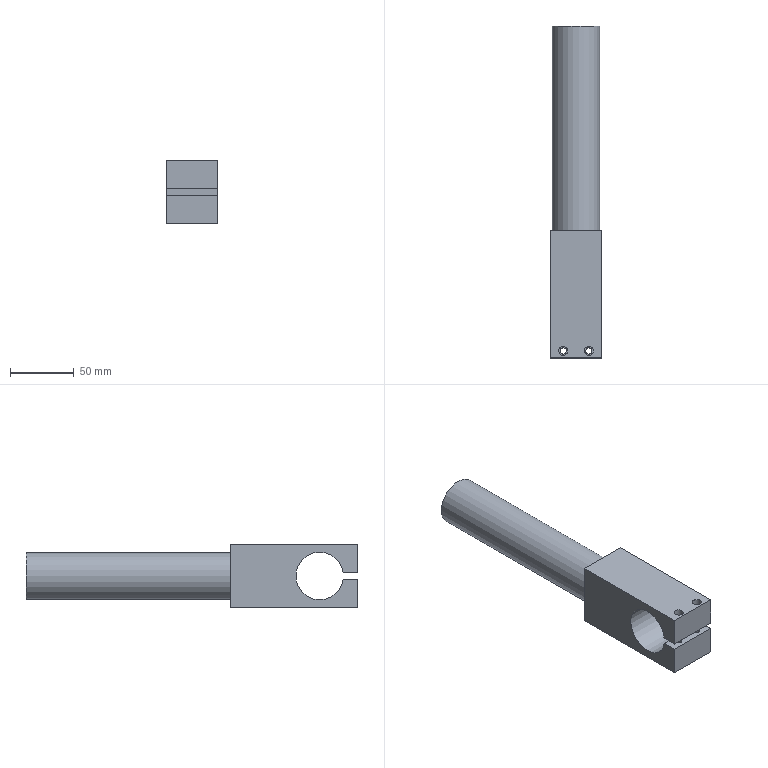Part | STEP file | SN10_010_001_SUPORTE | 1 solid | 16 faces | box 40 x 260 x 50 mm | volume 323681 mm3 | plane 10 | cylinder 6 | commonest cylinder face diameters 4.917 x2 7 x2 37 x1 37.2 x1
STEP:
#1=CARTESIAN_POINT('',(0.,0.,0.));
#2=DIRECTION('',(0.,0.,1.));
#3=DIRECTION('',(1.,0.,0.));
#4=AXIS2_PLACEMENT_3D('',#1,#2,#3);
#5=CARTESIAN_POINT('',(6.928,-22.822,2.5));
#6=VERTEX_POINT('',#5);
#7=CARTESIAN_POINT('',(10.,-24.5,2.5));
#8=DIRECTION('',(0.,0.,-1.));
#9=DIRECTION('',(1.,0.,0.));
#10=AXIS2_PLACEMENT_3D('',#7,#8,#9);
#11=CIRCLE('',#10,3.5);
#12=CARTESIAN_POINT('',(10.,-24.5,24.9));
#13=DIRECTION('',(0.,0.,-1.));
#14=DIRECTION('',(0.8776,-0.4794,0.));
#15=AXIS2_PLACEMENT_3D('',#12,#13,#14);
#16=CYLINDRICAL_SURFACE('',#15,3.5);
#17=CARTESIAN_POINT('',(-0.5,22.4));
#18=DIRECTION('',(1.,0.));
#19=VECTOR('',#18,1.);
#20=LINE('',#17,#19);
#21=(GEOMETRIC_REPRESENTATION_CONTEXT(2)PARAMETRIC_REPRESENTATION_CONTEXT()REPRESENTATION_CONTEXT('',''));
#22=DEFINITIONAL_REPRESENTATION('',(#20),#21);
#23=PCURVE('',#16,#22);
#24=CARTESIAN_POINT('',(20.,-30.,2.5));
#25=DIRECTION('',(0.,0.,1.));
#26=DIRECTION('',(1.,0.,0.));
#27=AXIS2_PLACEMENT_3D('',#24,#25,#26);
#28=PLANE('',#27);
#29=CARTESIAN_POINT('',(-6.5,5.5));
#30=CARTESIAN_POINT('',(-6.5,-0.5622));
#31=CARTESIAN_POINT('',(-11.75,2.469));
#32=CARTESIAN_POINT('',(-17.,5.5));
#33=CARTESIAN_POINT('',(-11.75,8.531));
#34=CARTESIAN_POINT('',(-6.5,11.562));
#35=CARTESIAN_POINT('',(-6.5,5.5));
#36=(BOUNDED_CURVE()B_SPLINE_CURVE(2,(#29,#30,#31,#32,#33,#34,#35),.UNSPECIFIED.,.T.,.F.)B_SPLINE_CURVE_WITH_KNOTS((1,2,2,2,2,1),(-2.094,0.,2.094,4.189,6.283,8.378),.UNSPECIFIED.)CURVE()GEOMETRIC_REPRESENTATION_ITEM()RATIONAL_B_SPLINE_CURVE((1.,0.5,1.,0.5,1.,0.5,1.))REPRESENTATION_ITEM(''));
#37=(GEOMETRIC_REPRESENTATION_CONTEXT(2)PARAMETRIC_REPRESENTATION_CONTEXT()REPRESENTATION_CONTEXT('',''));
#38=DEFINITIONAL_REPRESENTATION('',(#36),#37);
#39=PCURVE('',#28,#38);
#40=SURFACE_CURVE('',#11,(#23,#39),.PCURVE_S1.);
#41=EDGE_CURVE('',#6,#6,#40,.T.);
#42=ORIENTED_EDGE('',*,*,#41,.F.);
#43=CARTESIAN_POINT('',(6.928,-22.822,25.));
#44=VERTEX_POINT('',#43);
#45=CARTESIAN_POINT('',(6.928,-22.822,25.));
#46=CARTESIAN_POINT('',(6.928,-22.822,2.5));
#47=B_SPLINE_CURVE_WITH_KNOTS('',1,(#45,#46),.UNSPECIFIED.,.F.,.F.,(2,2),(-0.1,22.4),.PIECEWISE_BEZIER_KNOTS.);
#48=CARTESIAN_POINT('',(3.142,0.));
#49=DIRECTION('',(0.,1.));
#50=VECTOR('',#49,1.);
#51=LINE('',#48,#50);
#52=(GEOMETRIC_REPRESENTATION_CONTEXT(2)PARAMETRIC_REPRESENTATION_CONTEXT()REPRESENTATION_CONTEXT('',''));
#53=DEFINITIONAL_REPRESENTATION('',(#51),#52);
#54=PCURVE('',#16,#53);
#55=CARTESIAN_POINT('',(9.425,0.));
#56=DIRECTION('',(0.,1.));
#57=VECTOR('',#56,1.);
#58=LINE('',#55,#57);
#59=(GEOMETRIC_REPRESENTATION_CONTEXT(2)PARAMETRIC_REPRESENTATION_CONTEXT()REPRESENTATION_CONTEXT('',''));
#60=DEFINITIONAL_REPRESENTATION('',(#58),#59);
#61=PCURVE('',#16,#60);
#62=SEAM_CURVE('',#47,(#54,#61),.PCURVE_S1.);
#63=EDGE_CURVE('',#44,#6,#62,.T.);
#64=ORIENTED_EDGE('',*,*,#63,.F.);
#65=CARTESIAN_POINT('',(10.,-24.5,25.));
#66=DIRECTION('',(0.,0.,-1.));
#67=DIRECTION('',(1.,0.,0.));
#68=AXIS2_PLACEMENT_3D('',#65,#66,#67);
#69=CIRCLE('',#68,3.5);
#70=CARTESIAN_POINT('',(-0.5,-0.1));
#71=DIRECTION('',(1.,0.));
#72=VECTOR('',#71,1.);
#73=LINE('',#70,#72);
#74=(GEOMETRIC_REPRESENTATION_CONTEXT(2)PARAMETRIC_REPRESENTATION_CONTEXT()REPRESENTATION_CONTEXT('',''));
#75=DEFINITIONAL_REPRESENTATION('',(#73),#74);
#76=PCURVE('',#16,#75);
#77=CARTESIAN_POINT('',(0.,-30.,25.));
#78=DIRECTION('',(0.,0.,-1.));
#79=DIRECTION('',(-1.,0.,0.));
#80=AXIS2_PLACEMENT_3D('',#77,#78,#79);
#81=PLANE('',#80);
#82=CARTESIAN_POINT('',(-10.,5.5));
#83=DIRECTION('',(-1.,0.));
#84=AXIS2_PLACEMENT_2D('',#82,#83);
#85=CIRCLE('',#84,3.5);
#86=(GEOMETRIC_REPRESENTATION_CONTEXT(2)PARAMETRIC_REPRESENTATION_CONTEXT()REPRESENTATION_CONTEXT('',''));
#87=DEFINITIONAL_REPRESENTATION('',(#85),#86);
#88=PCURVE('',#81,#87);
#89=SURFACE_CURVE('',#69,(#76,#88),.PCURVE_S1.);
#90=EDGE_CURVE('',#44,#44,#89,.T.);
#91=ORIENTED_EDGE('',*,*,#90,.T.);
#92=ORIENTED_EDGE('',*,*,#63,.T.);
#93=EDGE_LOOP('',(#42,#64,#91,#92));
#94=FACE_BOUND('',#93,.F.);
#95=ADVANCED_FACE('',(#94),#16,.F.);
#96=CARTESIAN_POINT('',(20.,-30.,25.));
#97=VERTEX_POINT('',#96);
#98=CARTESIAN_POINT('',(20.,-30.,2.5));
#99=VERTEX_POINT('',#98);
#100=CARTESIAN_POINT('',(20.,-30.,25.));
#101=DIRECTION('',(0.,0.,-1.));
#102=VECTOR('',#101,1.);
#103=LINE('',#100,#102);
#104=CARTESIAN_POINT('',(0.,-30.,25.));
#105=DIRECTION('',(0.,-1.,0.));
#106=DIRECTION('',(0.,0.,-1.));
#107=AXIS2_PLACEMENT_3D('',#104,#105,#106);
#108=PLANE('',#107);
#109=CARTESIAN_POINT('',(0.,20.));
#110=DIRECTION('',(1.,0.));
#111=VECTOR('',#110,1.);
#112=LINE('',#109,#111);
#113=(GEOMETRIC_REPRESENTATION_CONTEXT(2)PARAMETRIC_REPRESENTATION_CONTEXT()REPRESENTATION_CONTEXT('',''));
#114=DEFINITIONAL_REPRESENTATION('',(#112),#113);
#115=PCURVE('',#108,#114);
#116=CARTESIAN_POINT('',(20.,0.,0.));
#117=DIRECTION('',(1.,0.,0.));
#118=DIRECTION('',(0.,0.,-1.));
#119=AXIS2_PLACEMENT_3D('',#116,#117,#118);
#120=PLANE('',#119);
#121=CARTESIAN_POINT('',(-25.,-30.));
#122=DIRECTION('',(1.,0.));
#123=VECTOR('',#122,1.);
#124=LINE('',#121,#123);
#125=(GEOMETRIC_REPRESENTATION_CONTEXT(2)PARAMETRIC_REPRESENTATION_CONTEXT()REPRESENTATION_CONTEXT('',''));
#126=DEFINITIONAL_REPRESENTATION('',(#124),#125);
#127=PCURVE('',#120,#126);
#128=SURFACE_CURVE('',#103,(#115,#127),.PCURVE_S1.);
#129=EDGE_CURVE('',#97,#99,#128,.T.);
#130=ORIENTED_EDGE('',*,*,#129,.F.);
#131=CARTESIAN_POINT('',(-20.,-30.,25.));
#132=VERTEX_POINT('',#131);
#133=CARTESIAN_POINT('',(-20.,-30.,25.));
#134=DIRECTION('',(1.,0.,0.));
#135=VECTOR('',#134,1.);
#136=LINE('',#133,#135);
#137=CARTESIAN_POINT('',(0.,-20.));
#138=DIRECTION('',(0.,1.));
#139=VECTOR('',#138,1.);
#140=LINE('',#137,#139);
#141=(GEOMETRIC_REPRESENTATION_CONTEXT(2)PARAMETRIC_REPRESENTATION_CONTEXT()REPRESENTATION_CONTEXT('',''));
#142=DEFINITIONAL_REPRESENTATION('',(#140),#141);
#143=PCURVE('',#108,#142);
#144=CARTESIAN_POINT('',(20.,0.));
#145=DIRECTION('',(-1.,0.));
#146=VECTOR('',#145,1.);
#147=LINE('',#144,#146);
#148=(GEOMETRIC_REPRESENTATION_CONTEXT(2)PARAMETRIC_REPRESENTATION_CONTEXT()REPRESENTATION_CONTEXT('',''));
#149=DEFINITIONAL_REPRESENTATION('',(#147),#148);
#150=PCURVE('',#81,#149);
#151=SURFACE_CURVE('',#136,(#143,#150),.PCURVE_S1.);
#152=EDGE_CURVE('',#132,#97,#151,.T.);
#153=ORIENTED_EDGE('',*,*,#152,.F.);
#154=CARTESIAN_POINT('',(-20.,-30.,2.5));
#155=VERTEX_POINT('',#154);
#156=CARTESIAN_POINT('',(-20.,-30.,25.));
#157=DIRECTION('',(0.,0.,-1.));
#158=VECTOR('',#157,1.);
#159=LINE('',#156,#158);
#160=CARTESIAN_POINT('',(0.,-20.));
#161=DIRECTION('',(1.,0.));
#162=VECTOR('',#161,1.);
#163=LINE('',#160,#162);
#164=(GEOMETRIC_REPRESENTATION_CONTEXT(2)PARAMETRIC_REPRESENTATION_CONTEXT()REPRESENTATION_CONTEXT('',''));
#165=DEFINITIONAL_REPRESENTATION('',(#163),#164);
#166=PCURVE('',#108,#165);
#167=CARTESIAN_POINT('',(-20.,0.,0.));
#168=DIRECTION('',(1.,0.,0.));
#169=DIRECTION('',(0.,0.,-1.));
#170=AXIS2_PLACEMENT_3D('',#167,#168,#169);
#171=PLANE('',#170);
#172=CARTESIAN_POINT('',(-25.,-30.));
#173=DIRECTION('',(1.,0.));
#174=VECTOR('',#173,1.);
#175=LINE('',#172,#174);
#176=(GEOMETRIC_REPRESENTATION_CONTEXT(2)PARAMETRIC_REPRESENTATION_CONTEXT()REPRESENTATION_CONTEXT('',''));
#177=DEFINITIONAL_REPRESENTATION('',(#175),#176);
#178=PCURVE('',#171,#177);
#179=SURFACE_CURVE('',#159,(#166,#178),.PCURVE_S1.);
#180=EDGE_CURVE('',#132,#155,#179,.T.);
#181=ORIENTED_EDGE('',*,*,#180,.T.);
#182=CARTESIAN_POINT('',(20.,-30.,2.5));
#183=DIRECTION('',(-1.,0.,0.));
#184=VECTOR('',#183,1.);
#185=LINE('',#182,#184);
#186=CARTESIAN_POINT('',(22.5,20.));
#187=DIRECTION('',(0.,-1.));
#188=VECTOR('',#187,1.);
#189=LINE('',#186,#188);
#190=(GEOMETRIC_REPRESENTATION_CONTEXT(2)PARAMETRIC_REPRESENTATION_CONTEXT()REPRESENTATION_CONTEXT('',''));
#191=DEFINITIONAL_REPRESENTATION('',(#189),#190);
#192=PCURVE('',#108,#191);
#193=CARTESIAN_POINT('',(0.,0.));
#194=DIRECTION('',(-1.,0.));
#195=VECTOR('',#194,1.);
#196=LINE('',#193,#195);
#197=(GEOMETRIC_REPRESENTATION_CONTEXT(2)PARAMETRIC_REPRESENTATION_CONTEXT()REPRESENTATION_CONTEXT('',''));
#198=DEFINITIONAL_REPRESENTATION('',(#196),#197);
#199=PCURVE('',#28,#198);
#200=SURFACE_CURVE('',#185,(#192,#199),.PCURVE_S1.);
#201=EDGE_CURVE('',#99,#155,#200,.T.);
#202=ORIENTED_EDGE('',*,*,#201,.F.);
#203=EDGE_LOOP('',(#130,#153,#181,#202));
#204=FACE_BOUND('',#203,.T.);
#205=ADVANCED_FACE('',(#204),#108,.T.);
#206=CARTESIAN_POINT('',(20.,-30.,-2.5));
#207=VERTEX_POINT('',#206);
#208=CARTESIAN_POINT('',(20.,-30.,-25.));
#209=VERTEX_POINT('',#208);
#210=CARTESIAN_POINT('',(20.,-30.,-2.5));
#211=DIRECTION('',(0.,0.,-1.));
#212=VECTOR('',#211,1.);
#213=LINE('',#210,#212);
#214=CARTESIAN_POINT('',(2.5,-30.));
#215=DIRECTION('',(1.,0.));
#216=VECTOR('',#215,1.);
#217=LINE('',#214,#216);
#218=(GEOMETRIC_REPRESENTATION_CONTEXT(2)PARAMETRIC_REPRESENTATION_CONTEXT()REPRESENTATION_CONTEXT('',''));
#219=DEFINITIONAL_REPRESENTATION('',(#217),#218);
#220=PCURVE('',#120,#219);
#221=CARTESIAN_POINT('',(0.,-30.,25.));
#222=DIRECTION('',(0.,-1.,0.));
#223=DIRECTION('',(0.,0.,-1.));
#224=AXIS2_PLACEMENT_3D('',#221,#222,#223);
#225=PLANE('',#224);
#226=CARTESIAN_POINT('',(27.5,20.));
#227=DIRECTION('',(1.,0.));
#228=VECTOR('',#227,1.);
#229=LINE('',#226,#228);
#230=(GEOMETRIC_REPRESENTATION_CONTEXT(2)PARAMETRIC_REPRESENTATION_CONTEXT()REPRESENTATION_CONTEXT('',''));
#231=DEFINITIONAL_REPRESENTATION('',(#229),#230);
#232=PCURVE('',#225,#231);
#233=SURFACE_CURVE('',#213,(#220,#232),.PCURVE_S1.);
#234=EDGE_CURVE('',#207,#209,#233,.T.);
#235=ORIENTED_EDGE('',*,*,#234,.T.);
#236=CARTESIAN_POINT('',(20.,70.,-25.));
#237=VERTEX_POINT('',#236);
#238=CARTESIAN_POINT('',(20.,70.,-25.));
#239=DIRECTION('',(0.,-1.,0.));
#240=VECTOR('',#239,1.);
#241=LINE('',#238,#240);
#242=CARTESIAN_POINT('',(25.,70.));
#243=DIRECTION('',(0.,-1.));
#244=VECTOR('',#243,1.);
#245=LINE('',#242,#244);
#246=(GEOMETRIC_REPRESENTATION_CONTEXT(2)PARAMETRIC_REPRESENTATION_CONTEXT()REPRESENTATION_CONTEXT('',''));
#247=DEFINITIONAL_REPRESENTATION('',(#245),#246);
#248=PCURVE('',#120,#247);
#249=CARTESIAN_POINT('',(0.,70.,-25.));
#250=DIRECTION('',(0.,0.,1.));
#251=DIRECTION('',(1.,0.,0.));
#252=AXIS2_PLACEMENT_3D('',#249,#250,#251);
#253=PLANE('',#252);
#254=CARTESIAN_POINT('',(20.,0.));
#255=DIRECTION('',(0.,-1.));
#256=VECTOR('',#255,1.);
#257=LINE('',#254,#256);
#258=(GEOMETRIC_REPRESENTATION_CONTEXT(2)PARAMETRIC_REPRESENTATION_CONTEXT()REPRESENTATION_CONTEXT('',''));
#259=DEFINITIONAL_REPRESENTATION('',(#257),#258);
#260=PCURVE('',#253,#259);
#261=SURFACE_CURVE('',#241,(#248,#260),.PCURVE_S1.);
#262=EDGE_CURVE('',#237,#209,#261,.T.);
#263=ORIENTED_EDGE('',*,*,#262,.F.);
#264=CARTESIAN_POINT('',(20.,70.,25.));
#265=VERTEX_POINT('',#264);
#266=CARTESIAN_POINT('',(20.,70.,-25.));
#267=DIRECTION('',(0.,0.,1.));
#268=VECTOR('',#267,1.);
#269=LINE('',#266,#268);
#270=CARTESIAN_POINT('',(25.,70.));
#271=DIRECTION('',(-1.,0.));
#272=VECTOR('',#271,1.);
#273=LINE('',#270,#272);
#274=(GEOMETRIC_REPRESENTATION_CONTEXT(2)PARAMETRIC_REPRESENTATION_CONTEXT()REPRESENTATION_CONTEXT('',''));
#275=DEFINITIONAL_REPRESENTATION('',(#273),#274);
#276=PCURVE('',#120,#275);
#277=CARTESIAN_POINT('',(0.,70.,-25.));
#278=DIRECTION('',(0.,1.,0.));
#279=DIRECTION('',(0.,0.,1.));
#280=AXIS2_PLACEMENT_3D('',#277,#278,#279);
#281=PLANE('',#280);
#282=CARTESIAN_POINT('',(0.,20.));
#283=DIRECTION('',(1.,0.));
#284=VECTOR('',#283,1.);
#285=LINE('',#282,#284);
#286=(GEOMETRIC_REPRESENTATION_CONTEXT(2)PARAMETRIC_REPRESENTATION_CONTEXT()REPRESENTATION_CONTEXT('',''));
#287=DEFINITIONAL_REPRESENTATION('',(#285),#286);
#288=PCURVE('',#281,#287);
#289=SURFACE_CURVE('',#269,(#276,#288),.PCURVE_S1.);
#290=EDGE_CURVE('',#237,#265,#289,.T.);
#291=ORIENTED_EDGE('',*,*,#290,.T.);
#292=CARTESIAN_POINT('',(20.,-30.,25.));
#293=DIRECTION('',(0.,1.,0.));
#294=VECTOR('',#293,1.);
#295=LINE('',#292,#294);
#296=CARTESIAN_POINT('',(-25.,-30.));
#297=DIRECTION('',(0.,1.));
#298=VECTOR('',#297,1.);
#299=LINE('',#296,#298);
#300=(GEOMETRIC_REPRESENTATION_CONTEXT(2)PARAMETRIC_REPRESENTATION_CONTEXT()REPRESENTATION_CONTEXT('',''));
#301=DEFINITIONAL_REPRESENTATION('',(#299),#300);
#302=PCURVE('',#120,#301);
#303=CARTESIAN_POINT('',(-20.,0.));
#304=DIRECTION('',(0.,1.));
#305=VECTOR('',#304,1.);
#306=LINE('',#303,#305);
#307=(GEOMETRIC_REPRESENTATION_CONTEXT(2)PARAMETRIC_REPRESENTATION_CONTEXT()REPRESENTATION_CONTEXT('',''));
#308=DEFINITIONAL_REPRESENTATION('',(#306),#307);
#309=PCURVE('',#81,#308);
#310=SURFACE_CURVE('',#295,(#302,#309),.PCURVE_S1.);
#311=EDGE_CURVE('',#97,#265,#310,.T.);
#312=ORIENTED_EDGE('',*,*,#311,.F.);
#313=ORIENTED_EDGE('',*,*,#129,.T.);
#314=CARTESIAN_POINT('',(20.,-18.431,2.5));
#315=VERTEX_POINT('',#314);
#316=CARTESIAN_POINT('',(20.,-30.,2.5));
#317=DIRECTION('',(0.,1.,0.));
#318=VECTOR('',#317,1.);
#319=LINE('',#316,#318);
#320=CARTESIAN_POINT('',(-2.5,-30.));
#321=DIRECTION('',(0.,1.));
#322=VECTOR('',#321,1.);
#323=LINE('',#320,#322);
#324=(GEOMETRIC_REPRESENTATION_CONTEXT(2)PARAMETRIC_REPRESENTATION_CONTEXT()REPRESENTATION_CONTEXT('',''));
#325=DEFINITIONAL_REPRESENTATION('',(#323),#324);
#326=PCURVE('',#120,#325);
#327=CARTESIAN_POINT('',(0.,0.));
#328=DIRECTION('',(0.,1.));
#329=VECTOR('',#328,1.);
#330=LINE('',#327,#329);
#331=(GEOMETRIC_REPRESENTATION_CONTEXT(2)PARAMETRIC_REPRESENTATION_CONTEXT()REPRESENTATION_CONTEXT('',''));
#332=DEFINITIONAL_REPRESENTATION('',(#330),#331);
#333=PCURVE('',#28,#332);
#334=SURFACE_CURVE('',#319,(#326,#333),.PCURVE_S1.);
#335=EDGE_CURVE('',#99,#315,#334,.T.);
#336=ORIENTED_EDGE('',*,*,#335,.T.);
#337=CARTESIAN_POINT('',(20.,-18.431,-2.5));
#338=VERTEX_POINT('',#337);
#339=CARTESIAN_POINT('',(20.,0.,0.));
#340=DIRECTION('',(1.,0.,0.));
#341=DIRECTION('',(0.,1.,0.));
#342=AXIS2_PLACEMENT_3D('',#339,#340,#341);
#343=CIRCLE('',#342,18.6);
#344=CARTESIAN_POINT('',(0.,0.));
#345=DIRECTION('',(0.,1.));
#346=AXIS2_PLACEMENT_2D('',#344,#345);
#347=CIRCLE('',#346,18.6);
#348=(GEOMETRIC_REPRESENTATION_CONTEXT(2)PARAMETRIC_REPRESENTATION_CONTEXT()REPRESENTATION_CONTEXT('',''));
#349=DEFINITIONAL_REPRESENTATION('',(#347),#348);
#350=PCURVE('',#120,#349);
#351=CARTESIAN_POINT('',(19.9,0.,0.));
#352=DIRECTION('',(-1.,0.,0.));
#353=DIRECTION('',(0.,0.8776,-0.4794));
#354=AXIS2_PLACEMENT_3D('',#351,#352,#353);
#355=CYLINDRICAL_SURFACE('',#354,18.6);
#356=CARTESIAN_POINT('',(12.066,-0.1));
#357=DIRECTION('',(-1.,0.));
#358=VECTOR('',#357,1.);
#359=LINE('',#356,#358);
#360=(GEOMETRIC_REPRESENTATION_CONTEXT(2)PARAMETRIC_REPRESENTATION_CONTEXT()REPRESENTATION_CONTEXT('',''));
#361=DEFINITIONAL_REPRESENTATION('',(#359),#360);
#362=PCURVE('',#355,#361);
#363=SURFACE_CURVE('',#343,(#350,#362),.PCURVE_S1.);
#364=EDGE_CURVE('',#338,#315,#363,.T.);
#365=ORIENTED_EDGE('',*,*,#364,.F.);
#366=CARTESIAN_POINT('',(20.,-18.431,-2.5));
#367=DIRECTION('',(0.,-1.,0.));
#368=VECTOR('',#367,1.);
#369=LINE('',#366,#368);
#370=CARTESIAN_POINT('',(2.5,-18.431));
#371=DIRECTION('',(0.,-1.));
#372=VECTOR('',#371,1.);
#373=LINE('',#370,#372);
#374=(GEOMETRIC_REPRESENTATION_CONTEXT(2)PARAMETRIC_REPRESENTATION_CONTEXT()REPRESENTATION_CONTEXT('',''));
#375=DEFINITIONAL_REPRESENTATION('',(#373),#374);
#376=PCURVE('',#120,#375);
#377=CARTESIAN_POINT('',(20.,-18.431,-2.5));
#378=DIRECTION('',(0.,0.,-1.));
#379=DIRECTION('',(-1.,0.,0.));
#380=AXIS2_PLACEMENT_3D('',#377,#378,#379);
#381=PLANE('',#380);
#382=CARTESIAN_POINT('',(0.,0.));
#383=DIRECTION('',(0.,-1.));
#384=VECTOR('',#383,1.);
#385=LINE('',#382,#384);
#386=(GEOMETRIC_REPRESENTATION_CONTEXT(2)PARAMETRIC_REPRESENTATION_CONTEXT()REPRESENTATION_CONTEXT('',''));
#387=DEFINITIONAL_REPRESENTATION('',(#385),#386);
#388=PCURVE('',#381,#387);
#389=SURFACE_CURVE('',#369,(#376,#388),.PCURVE_S1.);
#390=EDGE_CURVE('',#338,#207,#389,.T.);
#391=ORIENTED_EDGE('',*,*,#390,.T.);
#392=EDGE_LOOP('',(#235,#263,#291,#312,#313,#336,#365,#391));
#393=FACE_BOUND('',#392,.T.);
#394=ADVANCED_FACE('',(#393),#120,.T.);
#395=CARTESIAN_POINT('',(-20.,-30.,-2.5));
#396=VERTEX_POINT('',#395);
#397=CARTESIAN_POINT('',(-20.,-18.431,-2.5));
#398=VERTEX_POINT('',#397);
#399=CARTESIAN_POINT('',(-20.,-30.,-2.5));
#400=DIRECTION('',(0.,1.,0.));
#401=VECTOR('',#400,1.);
#402=LINE('',#399,#401);
#403=CARTESIAN_POINT('',(2.5,-30.));
#404=DIRECTION('',(0.,1.));
#405=VECTOR('',#404,1.);
#406=LINE('',#403,#405);
#407=(GEOMETRIC_REPRESENTATION_CONTEXT(2)PARAMETRIC_REPRESENTATION_CONTEXT()REPRESENTATION_CONTEXT('',''));
#408=DEFINITIONAL_REPRESENTATION('',(#406),#407);
#409=PCURVE('',#171,#408);
#410=CARTESIAN_POINT('',(40.,-11.569));
#411=DIRECTION('',(0.,1.));
#412=VECTOR('',#411,1.);
#413=LINE('',#410,#412);
#414=(GEOMETRIC_REPRESENTATION_CONTEXT(2)PARAMETRIC_REPRESENTATION_CONTEXT()REPRESENTATION_CONTEXT('',''));
#415=DEFINITIONAL_REPRESENTATION('',(#413),#414);
#416=PCURVE('',#381,#415);
#417=SURFACE_CURVE('',#402,(#409,#416),.PCURVE_S1.);
#418=EDGE_CURVE('',#396,#398,#417,.T.);
#419=ORIENTED_EDGE('',*,*,#418,.T.);
#420=CARTESIAN_POINT('',(-20.,-18.431,2.5));
#421=VERTEX_POINT('',#420);
#422=CARTESIAN_POINT('',(-20.,0.,0.));
#423=DIRECTION('',(1.,0.,0.));
#424=DIRECTION('',(0.,1.,0.));
#425=AXIS2_PLACEMENT_3D('',#422,#423,#424);
#426=CIRCLE('',#425,18.6);
#427=CARTESIAN_POINT('',(0.,0.));
#428=DIRECTION('',(0.,1.));
#429=AXIS2_PLACEMENT_2D('',#427,#428);
#430=CIRCLE('',#429,18.6);
#431=(GEOMETRIC_REPRESENTATION_CONTEXT(2)PARAMETRIC_REPRESENTATION_CONTEXT()REPRESENTATION_CONTEXT('',''));
#432=DEFINITIONAL_REPRESENTATION('',(#430),#431);
#433=PCURVE('',#171,#432);
#434=CARTESIAN_POINT('',(12.066,39.9));
#435=DIRECTION('',(-1.,0.));
#436=VECTOR('',#435,1.);
#437=LINE('',#434,#436);
#438=(GEOMETRIC_REPRESENTATION_CONTEXT(2)PARAMETRIC_REPRESENTATION_CONTEXT()REPRESENTATION_CONTEXT('',''));
#439=DEFINITIONAL_REPRESENTATION('',(#437),#438);
#440=PCURVE('',#355,#439);
#441=SURFACE_CURVE('',#426,(#433,#440),.PCURVE_S1.);
#442=EDGE_CURVE('',#398,#421,#441,.T.);
#443=ORIENTED_EDGE('',*,*,#442,.T.);
#444=CARTESIAN_POINT('',(-20.,-30.,2.5));
#445=DIRECTION('',(0.,1.,0.));
#446=VECTOR('',#445,1.);
#447=LINE('',#444,#446);
#448=CARTESIAN_POINT('',(-2.5,-30.));
#449=DIRECTION('',(0.,1.));
#450=VECTOR('',#449,1.);
#451=LINE('',#448,#450);
#452=(GEOMETRIC_REPRESENTATION_CONTEXT(2)PARAMETRIC_REPRESENTATION_CONTEXT()REPRESENTATION_CONTEXT('',''));
#453=DEFINITIONAL_REPRESENTATION('',(#451),#452);
#454=PCURVE('',#171,#453);
#455=CARTESIAN_POINT('',(-40.,0.));
#456=DIRECTION('',(0.,1.));
#457=VECTOR('',#456,1.);
#458=LINE('',#455,#457);
#459=(GEOMETRIC_REPRESENTATION_CONTEXT(2)PARAMETRIC_REPRESENTATION_CONTEXT()REPRESENTATION_CONTEXT('',''));
#460=DEFINITIONAL_REPRESENTATION('',(#458),#459);
#461=PCURVE('',#28,#460);
#462=SURFACE_CURVE('',#447,(#454,#461),.PCURVE_S1.);
#463=EDGE_CURVE('',#155,#421,#462,.T.);
#464=ORIENTED_EDGE('',*,*,#463,.F.);
#465=ORIENTED_EDGE('',*,*,#180,.F.);
#466=CARTESIAN_POINT('',(-20.,70.,25.));
#467=VERTEX_POINT('',#466);
#468=CARTESIAN_POINT('',(-20.,-30.,25.));
#469=DIRECTION('',(0.,1.,0.));
#470=VECTOR('',#469,1.);
#471=LINE('',#468,#470);
#472=CARTESIAN_POINT('',(-25.,-30.));
#473=DIRECTION('',(0.,1.));
#474=VECTOR('',#473,1.);
#475=LINE('',#472,#474);
#476=(GEOMETRIC_REPRESENTATION_CONTEXT(2)PARAMETRIC_REPRESENTATION_CONTEXT()REPRESENTATION_CONTEXT('',''));
#477=DEFINITIONAL_REPRESENTATION('',(#475),#476);
#478=PCURVE('',#171,#477);
#479=CARTESIAN_POINT('',(20.,0.));
#480=DIRECTION('',(0.,1.));
#481=VECTOR('',#480,1.);
#482=LINE('',#479,#481);
#483=(GEOMETRIC_REPRESENTATION_CONTEXT(2)PARAMETRIC_REPRESENTATION_CONTEXT()REPRESENTATION_CONTEXT('',''));
#484=DEFINITIONAL_REPRESENTATION('',(#482),#483);
#485=PCURVE('',#81,#484);
#486=SURFACE_CURVE('',#471,(#478,#485),.PCURVE_S1.);
#487=EDGE_CURVE('',#132,#467,#486,.T.);
#488=ORIENTED_EDGE('',*,*,#487,.T.);
#489=CARTESIAN_POINT('',(-20.,70.,-25.));
#490=VERTEX_POINT('',#489);
#491=CARTESIAN_POINT('',(-20.,70.,-25.));
#492=DIRECTION('',(0.,0.,1.));
#493=VECTOR('',#492,1.);
#494=LINE('',#491,#493);
#495=CARTESIAN_POINT('',(25.,70.));
#496=DIRECTION('',(-1.,0.));
#497=VECTOR('',#496,1.);
#498=LINE('',#495,#497);
#499=(GEOMETRIC_REPRESENTATION_CONTEXT(2)PARAMETRIC_REPRESENTATION_CONTEXT()REPRESENTATION_CONTEXT('',''));
#500=DEFINITIONAL_REPRESENTATION('',(#498),#499);
#501=PCURVE('',#171,#500);
#502=CARTESIAN_POINT('',(0.,-20.));
#503=DIRECTION('',(1.,0.));
#504=VECTOR('',#503,1.);
#505=LINE('',#502,#504);
#506=(GEOMETRIC_REPRESENTATION_CONTEXT(2)PARAMETRIC_REPRESENTATION_CONTEXT()REPRESENTATION_CONTEXT('',''));
#507=DEFINITIONAL_REPRESENTATION('',(#505),#506);
#508=PCURVE('',#281,#507);
#509=SURFACE_CURVE('',#494,(#501,#508),.PCURVE_S1.);
#510=EDGE_CURVE('',#490,#467,#509,.T.);
#511=ORIENTED_EDGE('',*,*,#510,.F.);
#512=CARTESIAN_POINT('',(-20.,-30.,-25.));
#513=VERTEX_POINT('',#512);
#514=CARTESIAN_POINT('',(-20.,70.,-25.));
#515=DIRECTION('',(0.,-1.,0.));
#516=VECTOR('',#515,1.);
#517=LINE('',#514,#516);
#518=CARTESIAN_POINT('',(25.,70.));
#519=DIRECTION('',(0.,-1.));
#520=VECTOR('',#519,1.);
#521=LINE('',#518,#520);
#522=(GEOMETRIC_REPRESENTATION_CONTEXT(2)PARAMETRIC_REPRESENTATION_CONTEXT()REPRESENTATION_CONTEXT('',''));
#523=DEFINITIONAL_REPRESENTATION('',(#521),#522);
#524=PCURVE('',#171,#523);
#525=CARTESIAN_POINT('',(-20.,0.));
#526=DIRECTION('',(0.,-1.));
#527=VECTOR('',#526,1.);
#528=LINE('',#525,#527);
#529=(GEOMETRIC_REPRESENTATION_CONTEXT(2)PARAMETRIC_REPRESENTATION_CONTEXT()REPRESENTATION_CONTEXT('',''));
#530=DEFINITIONAL_REPRESENTATION('',(#528),#529);
#531=PCURVE('',#253,#530);
#532=SURFACE_CURVE('',#517,(#524,#531),.PCURVE_S1.);
#533=EDGE_CURVE('',#490,#513,#532,.T.);
#534=ORIENTED_EDGE('',*,*,#533,.T.);
#535=CARTESIAN_POINT('',(-20.,-30.,-2.5));
#536=DIRECTION('',(0.,0.,-1.));
#537=VECTOR('',#536,1.);
#538=LINE('',#535,#537);
#539=CARTESIAN_POINT('',(2.5,-30.));
#540=DIRECTION('',(1.,0.));
#541=VECTOR('',#540,1.);
#542=LINE('',#539,#541);
#543=(GEOMETRIC_REPRESENTATION_CONTEXT(2)PARAMETRIC_REPRESENTATION_CONTEXT()REPRESENTATION_CONTEXT('',''));
#544=DEFINITIONAL_REPRESENTATION('',(#542),#543);
#545=PCURVE('',#171,#544);
#546=CARTESIAN_POINT('',(27.5,-20.));
#547=DIRECTION('',(1.,0.));
#548=VECTOR('',#547,1.);
#549=LINE('',#546,#548);
#550=(GEOMETRIC_REPRESENTATION_CONTEXT(2)PARAMETRIC_REPRESENTATION_CONTEXT()REPRESENTATION_CONTEXT('',''));
#551=DEFINITIONAL_REPRESENTATION('',(#549),#550);
#552=PCURVE('',#225,#551);
#553=SURFACE_CURVE('',#538,(#545,#552),.PCURVE_S1.);
#554=EDGE_CURVE('',#396,#513,#553,.T.);
#555=ORIENTED_EDGE('',*,*,#554,.F.);
#556=EDGE_LOOP('',(#419,#443,#464,#465,#488,#511,#534,#555));
#557=FACE_BOUND('',#556,.T.);
#558=ADVANCED_FACE('',(#557),#171,.F.);
#559=CARTESIAN_POINT('',(-6.928,-26.178,2.5));
#560=VERTEX_POINT('',#559);
#561=CARTESIAN_POINT('',(-10.,-24.5,2.5));
#562=DIRECTION('',(0.,0.,-1.));
#563=DIRECTION('',(1.,0.,0.));
#564=AXIS2_PLACEMENT_3D('',#561,#562,#563);
#565=CIRCLE('',#564,3.5);
#566=CARTESIAN_POINT('',(-10.,-24.5,24.9));
#567=DIRECTION('',(0.,0.,-1.));
#568=DIRECTION('',(0.8776,-0.4794,0.));
#569=AXIS2_PLACEMENT_3D('',#566,#567,#568);
#570=CYLINDRICAL_SURFACE('',#569,3.5);
#571=CARTESIAN_POINT('',(-0.5,22.4));
#572=DIRECTION('',(1.,0.));
#573=VECTOR('',#572,1.);
#574=LINE('',#571,#573);
#575=(GEOMETRIC_REPRESENTATION_CONTEXT(2)PARAMETRIC_REPRESENTATION_CONTEXT()REPRESENTATION_CONTEXT('',''));
#576=DEFINITIONAL_REPRESENTATION('',(#574),#575);
#577=PCURVE('',#570,#576);
#578=CARTESIAN_POINT('',(-26.5,5.5));
#579=CARTESIAN_POINT('',(-26.5,-0.5622));
#580=CARTESIAN_POINT('',(-31.75,2.469));
#581=CARTESIAN_POINT('',(-37.,5.5));
#582=CARTESIAN_POINT('',(-31.75,8.531));
#583=CARTESIAN_POINT('',(-26.5,11.562));
#584=CARTESIAN_POINT('',(-26.5,5.5));
#585=(BOUNDED_CURVE()B_SPLINE_CURVE(2,(#578,#579,#580,#581,#582,#583,#584),.UNSPECIFIED.,.T.,.F.)B_SPLINE_CURVE_WITH_KNOTS((1,2,2,2,2,1),(-2.094,0.,2.094,4.189,6.283,8.378),.UNSPECIFIED.)CURVE()GEOMETRIC_REPRESENTATION_ITEM()RATIONAL_B_SPLINE_CURVE((1.,0.5,1.,0.5,1.,0.5,1.))REPRESENTATION_ITEM(''));
#586=(GEOMETRIC_REPRESENTATION_CONTEXT(2)PARAMETRIC_REPRESENTATION_CONTEXT()REPRESENTATION_CONTEXT('',''));
#587=DEFINITIONAL_REPRESENTATION('',(#585),#586);
#588=PCURVE('',#28,#587);
#589=SURFACE_CURVE('',#565,(#577,#588),.PCURVE_S1.);
#590=EDGE_CURVE('',#560,#560,#589,.T.);
#591=ORIENTED_EDGE('',*,*,#590,.F.);
#592=CARTESIAN_POINT('',(-6.928,-26.178,25.));
#593=VERTEX_POINT('',#592);
#594=CARTESIAN_POINT('',(-6.928,-26.178,25.));
#595=CARTESIAN_POINT('',(-6.928,-26.178,2.5));
#596=B_SPLINE_CURVE_WITH_KNOTS('',1,(#594,#595),.UNSPECIFIED.,.F.,.F.,(2,2),(-0.1,22.4),.PIECEWISE_BEZIER_KNOTS.);
#597=CARTESIAN_POINT('',(0.,0.));
#598=DIRECTION('',(0.,1.));
#599=VECTOR('',#598,1.);
#600=LINE('',#597,#599);
#601=(GEOMETRIC_REPRESENTATION_CONTEXT(2)PARAMETRIC_REPRESENTATION_CONTEXT()REPRESENTATION_CONTEXT('',''));
#602=DEFINITIONAL_REPRESENTATION('',(#600),#601);
#603=PCURVE('',#570,#602);
#604=CARTESIAN_POINT('',(6.283,0.));
#605=DIRECTION('',(0.,1.));
#606=VECTOR('',#605,1.);
#607=LINE('',#604,#606);
#608=(GEOMETRIC_REPRESENTATION_CONTEXT(2)PARAMETRIC_REPRESENTATION_CONTEXT()REPRESENTATION_CONTEXT('',''));
#609=DEFINITIONAL_REPRESENTATION('',(#607),#608);
#610=PCURVE('',#570,#609);
#611=SEAM_CURVE('',#596,(#603,#610),.PCURVE_S1.);
#612=EDGE_CURVE('',#593,#560,#611,.T.);
#613=ORIENTED_EDGE('',*,*,#612,.F.);
#614=CARTESIAN_POINT('',(-10.,-24.5,25.));
#615=DIRECTION('',(0.,0.,-1.));
#616=DIRECTION('',(1.,0.,0.));
#617=AXIS2_PLACEMENT_3D('',#614,#615,#616);
#618=CIRCLE('',#617,3.5);
#619=CARTESIAN_POINT('',(-0.5,-0.1));
#620=DIRECTION('',(1.,0.));
#621=VECTOR('',#620,1.);
#622=LINE('',#619,#621);
#623=(GEOMETRIC_REPRESENTATION_CONTEXT(2)PARAMETRIC_REPRESENTATION_CONTEXT()REPRESENTATION_CONTEXT('',''));
#624=DEFINITIONAL_REPRESENTATION('',(#622),#623);
#625=PCURVE('',#570,#624);
#626=CARTESIAN_POINT('',(10.,5.5));
#627=DIRECTION('',(-1.,0.));
#628=AXIS2_PLACEMENT_2D('',#626,#627);
#629=CIRCLE('',#628,3.5);
#630=(GEOMETRIC_REPRESENTATION_CONTEXT(2)PARAMETRIC_REPRESENTATION_CONTEXT()REPRESENTATION_CONTEXT('',''));
#631=DEFINITIONAL_REPRESENTATION('',(#629),#630);
#632=PCURVE('',#81,#631);
#633=SURFACE_CURVE('',#618,(#625,#632),.PCURVE_S1.);
#634=EDGE_CURVE('',#593,#593,#633,.T.);
#635=ORIENTED_EDGE('',*,*,#634,.T.);
#636=ORIENTED_EDGE('',*,*,#612,.T.);
#637=EDGE_LOOP('',(#591,#613,#635,#636));
#638=FACE_BOUND('',#637,.F.);
#639=ADVANCED_FACE('',(#638),#570,.F.);
#640=ORIENTED_EDGE('',*,*,#554,.T.);
#641=CARTESIAN_POINT('',(-20.,-30.,-25.));
#642=DIRECTION('',(1.,0.,0.));
#643=VECTOR('',#642,1.);
#644=LINE('',#641,#643);
#645=CARTESIAN_POINT('',(50.,-20.));
#646=DIRECTION('',(0.,1.));
#647=VECTOR('',#646,1.);
#648=LINE('',#645,#647);
#649=(GEOMETRIC_REPRESENTATION_CONTEXT(2)PARAMETRIC_REPRESENTATION_CONTEXT()REPRESENTATION_CONTEXT('',''));
#650=DEFINITIONAL_REPRESENTATION('',(#648),#649);
#651=PCURVE('',#225,#650);
#652=CARTESIAN_POINT('',(-20.,-100.));
#653=DIRECTION('',(1.,0.));
#654=VECTOR('',#653,1.);
#655=LINE('',#652,#654);
#656=(GEOMETRIC_REPRESENTATION_CONTEXT(2)PARAMETRIC_REPRESENTATION_CONTEXT()REPRESENTATION_CONTEXT('',''));
#657=DEFINITIONAL_REPRESENTATION('',(#655),#656);
#658=PCURVE('',#253,#657);
#659=SURFACE_CURVE('',#644,(#651,#658),.PCURVE_S1.);
#660=EDGE_CURVE('',#513,#209,#659,.T.);
#661=ORIENTED_EDGE('',*,*,#660,.T.);
#662=ORIENTED_EDGE('',*,*,#234,.F.);
#663=CARTESIAN_POINT('',(20.,-30.,-2.5));
#664=DIRECTION('',(-1.,0.,0.));
#665=VECTOR('',#664,1.);
#666=LINE('',#663,#665);
#667=CARTESIAN_POINT('',(27.5,20.));
#668=DIRECTION('',(0.,-1.));
#669=VECTOR('',#668,1.);
#670=LINE('',#667,#669);
#671=(GEOMETRIC_REPRESENTATION_CONTEXT(2)PARAMETRIC_REPRESENTATION_CONTEXT()REPRESENTATION_CONTEXT('',''));
#672=DEFINITIONAL_REPRESENTATION('',(#670),#671);
#673=PCURVE('',#225,#672);
#674=CARTESIAN_POINT('',(0.,-11.569));
#675=DIRECTION('',(1.,0.));
#676=VECTOR('',#675,1.);
#677=LINE('',#674,#676);
#678=(GEOMETRIC_REPRESENTATION_CONTEXT(2)PARAMETRIC_REPRESENTATION_CONTEXT()REPRESENTATION_CONTEXT('',''));
#679=DEFINITIONAL_REPRESENTATION('',(#677),#678);
#680=PCURVE('',#381,#679);
#681=SURFACE_CURVE('',#666,(#673,#680),.PCURVE_S1.);
#682=EDGE_CURVE('',#207,#396,#681,.T.);
#683=ORIENTED_EDGE('',*,*,#682,.T.);
#684=EDGE_LOOP('',(#640,#661,#662,#683));
#685=FACE_BOUND('',#684,.T.);
#686=ADVANCED_FACE('',(#685),#225,.T.);
#687=ORIENTED_EDGE('',*,*,#660,.F.);
#688=ORIENTED_EDGE('',*,*,#533,.F.);
#689=CARTESIAN_POINT('',(-20.,70.,-25.));
#690=DIRECTION('',(1.,0.,0.));
#691=VECTOR('',#690,1.);
#692=LINE('',#689,#691);
#693=CARTESIAN_POINT('',(-20.,0.));
#694=DIRECTION('',(1.,0.));
#695=VECTOR('',#694,1.);
#696=LINE('',#693,#695);
#697=(GEOMETRIC_REPRESENTATION_CONTEXT(2)PARAMETRIC_REPRESENTATION_CONTEXT()REPRESENTATION_CONTEXT('',''));
#698=DEFINITIONAL_REPRESENTATION('',(#696),#697);
#699=PCURVE('',#253,#698);
#700=CARTESIAN_POINT('',(0.,-20.));
#701=DIRECTION('',(0.,1.));
#702=VECTOR('',#701,1.);
#703=LINE('',#700,#702);
#704=(GEOMETRIC_REPRESENTATION_CONTEXT(2)PARAMETRIC_REPRESENTATION_CONTEXT()REPRESENTATION_CONTEXT('',''));
#705=DEFINITIONAL_REPRESENTATION('',(#703),#704);
#706=PCURVE('',#281,#705);
#707=SURFACE_CURVE('',#692,(#699,#706),.PCURVE_S1.);
#708=EDGE_CURVE('',#490,#237,#707,.T.);
#709=ORIENTED_EDGE('',*,*,#708,.T.);
#710=ORIENTED_EDGE('',*,*,#262,.T.);
#711=EDGE_LOOP('',(#687,#688,#709,#710));
#712=FACE_BOUND('',#711,.T.);
#713=CARTESIAN_POINT('',(7.842,-23.321,-25.));
#714=VERTEX_POINT('',#713);
#715=CARTESIAN_POINT('',(10.,-24.5,-25.));
#716=DIRECTION('',(0.,0.,1.));
#717=DIRECTION('',(1.,0.,0.));
#718=AXIS2_PLACEMENT_3D('',#715,#716,#717);
#719=CIRCLE('',#718,2.458);
#720=CARTESIAN_POINT('',(10.,-94.5));
#721=DIRECTION('',(1.,0.));
#722=AXIS2_PLACEMENT_2D('',#720,#721);
#723=CIRCLE('',#722,2.458);
#724=(GEOMETRIC_REPRESENTATION_CONTEXT(2)PARAMETRIC_REPRESENTATION_CONTEXT()REPRESENTATION_CONTEXT('',''));
#725=DEFINITIONAL_REPRESENTATION('',(#723),#724);
#726=PCURVE('',#253,#725);
#727=CARTESIAN_POINT('',(10.,-24.5,-2.6));
#728=DIRECTION('',(0.,0.,-1.));
#729=DIRECTION('',(0.8776,-0.4794,0.));
#730=AXIS2_PLACEMENT_3D('',#727,#728,#729);
#731=CYLINDRICAL_SURFACE('',#730,2.458);
#732=CARTESIAN_POINT('',(12.066,22.4));
#733=DIRECTION('',(-1.,0.));
#734=VECTOR('',#733,1.);
#735=LINE('',#732,#734);
#736=(GEOMETRIC_REPRESENTATION_CONTEXT(2)PARAMETRIC_REPRESENTATION_CONTEXT()REPRESENTATION_CONTEXT('',''));
#737=DEFINITIONAL_REPRESENTATION('',(#735),#736);
#738=PCURVE('',#731,#737);
#739=SURFACE_CURVE('',#719,(#726,#738),.PCURVE_S1.);
#740=EDGE_CURVE('',#714,#714,#739,.T.);
#741=ORIENTED_EDGE('',*,*,#740,.T.);
#742=EDGE_LOOP('',(#741));
#743=FACE_BOUND('',#742,.T.);
#744=CARTESIAN_POINT('',(-12.158,-23.321,-25.));
#745=VERTEX_POINT('',#744);
#746=CARTESIAN_POINT('',(-10.,-24.5,-25.));
#747=DIRECTION('',(0.,0.,1.));
#748=DIRECTION('',(1.,0.,0.));
#749=AXIS2_PLACEMENT_3D('',#746,#747,#748);
#750=CIRCLE('',#749,2.458);
#751=CARTESIAN_POINT('',(-10.,-94.5));
#752=DIRECTION('',(1.,0.));
#753=AXIS2_PLACEMENT_2D('',#751,#752);
#754=CIRCLE('',#753,2.458);
#755=(GEOMETRIC_REPRESENTATION_CONTEXT(2)PARAMETRIC_REPRESENTATION_CONTEXT()REPRESENTATION_CONTEXT('',''));
#756=DEFINITIONAL_REPRESENTATION('',(#754),#755);
#757=PCURVE('',#253,#756);
#758=CARTESIAN_POINT('',(-10.,-24.5,-2.6));
#759=DIRECTION('',(0.,0.,-1.));
#760=DIRECTION('',(0.8776,-0.4794,0.));
#761=AXIS2_PLACEMENT_3D('',#758,#759,#760);
#762=CYLINDRICAL_SURFACE('',#761,2.458);
#763=CARTESIAN_POINT('',(12.066,22.4));
#764=DIRECTION('',(-1.,0.));
#765=VECTOR('',#764,1.);
#766=LINE('',#763,#765);
#767=(GEOMETRIC_REPRESENTATION_CONTEXT(2)PARAMETRIC_REPRESENTATION_CONTEXT()REPRESENTATION_CONTEXT('',''));
#768=DEFINITIONAL_REPRESENTATION('',(#766),#767);
#769=PCURVE('',#762,#768);
#770=SURFACE_CURVE('',#750,(#757,#769),.PCURVE_S1.);
#771=EDGE_CURVE('',#745,#745,#770,.T.);
#772=ORIENTED_EDGE('',*,*,#771,.T.);
#773=EDGE_LOOP('',(#772));
#774=FACE_BOUND('',#773,.T.);
#775=ADVANCED_FACE('',(#712,#743,#774),#253,.F.);
#776=ORIENTED_EDGE('',*,*,#708,.F.);
#777=ORIENTED_EDGE('',*,*,#510,.T.);
#778=CARTESIAN_POINT('',(-20.,70.,25.));
#779=DIRECTION('',(1.,0.,0.));
#780=VECTOR('',#779,1.);
#781=LINE('',#778,#780);
#782=CARTESIAN_POINT('',(50.,-20.));
#783=DIRECTION('',(0.,1.));
#784=VECTOR('',#783,1.);
#785=LINE('',#782,#784);
#786=(GEOMETRIC_REPRESENTATION_CONTEXT(2)PARAMETRIC_REPRESENTATION_CONTEXT()REPRESENTATION_CONTEXT('',''));
#787=DEFINITIONAL_REPRESENTATION('',(#785),#786);
#788=PCURVE('',#281,#787);
#789=CARTESIAN_POINT('',(20.,100.));
#790=DIRECTION('',(-1.,0.));
#791=VECTOR('',#790,1.);
#792=LINE('',#789,#791);
#793=(GEOMETRIC_REPRESENTATION_CONTEXT(2)PARAMETRIC_REPRESENTATION_CONTEXT()REPRESENTATION_CONTEXT('',''));
#794=DEFINITIONAL_REPRESENTATION('',(#792),#793);
#795=PCURVE('',#81,#794);
#796=SURFACE_CURVE('',#781,(#788,#795),.PCURVE_S1.);
#797=EDGE_CURVE('',#467,#265,#796,.T.);
#798=ORIENTED_EDGE('',*,*,#797,.T.);
#799=ORIENTED_EDGE('',*,*,#290,.F.);
#800=EDGE_LOOP('',(#776,#777,#798,#799));
#801=FACE_BOUND('',#800,.T.);
#802=CARTESIAN_POINT('',(-18.5,70.,0.));
#803=VERTEX_POINT('',#802);
#804=CARTESIAN_POINT('',(0.,70.,0.));
#805=DIRECTION('',(0.,1.,0.));
#806=DIRECTION('',(1.,0.,0.));
#807=AXIS2_PLACEMENT_3D('',#804,#805,#806);
#808=CIRCLE('',#807,18.5);
#809=CARTESIAN_POINT('',(25.,0.));
#810=DIRECTION('',(0.,1.));
#811=AXIS2_PLACEMENT_2D('',#809,#810);
#812=CIRCLE('',#811,18.5);
#813=(GEOMETRIC_REPRESENTATION_CONTEXT(2)PARAMETRIC_REPRESENTATION_CONTEXT()REPRESENTATION_CONTEXT('',''));
#814=DEFINITIONAL_REPRESENTATION('',(#812),#813);
#815=PCURVE('',#281,#814);
#816=CARTESIAN_POINT('',(0.,150.,0.));
#817=DIRECTION('',(0.,1.,0.));
#818=DIRECTION('',(-1.,0.,0.));
#819=AXIS2_PLACEMENT_3D('',#816,#817,#818);
#820=CYLINDRICAL_SURFACE('',#819,18.5);
#821=CARTESIAN_POINT('',(-3.142,-80.));
#822=DIRECTION('',(1.,0.));
#823=VECTOR('',#822,1.);
#824=LINE('',#821,#823);
#825=(GEOMETRIC_REPRESENTATION_CONTEXT(2)PARAMETRIC_REPRESENTATION_CONTEXT()REPRESENTATION_CONTEXT('',''));
#826=DEFINITIONAL_REPRESENTATION('',(#824),#825);
#827=PCURVE('',#820,#826);
#828=SURFACE_CURVE('',#808,(#815,#827),.PCURVE_S1.);
#829=EDGE_CURVE('',#803,#803,#828,.T.);
#830=ORIENTED_EDGE('',*,*,#829,.F.);
#831=EDGE_LOOP('',(#830));
#832=FACE_BOUND('',#831,.T.);
#833=ADVANCED_FACE('',(#801,#832),#281,.T.);
#834=CARTESIAN_POINT('',(7.842,-23.321,-2.5));
#835=VERTEX_POINT('',#834);
#836=CARTESIAN_POINT('',(10.,-24.5,-2.5));
#837=DIRECTION('',(0.,0.,-1.));
#838=DIRECTION('',(1.,0.,0.));
#839=AXIS2_PLACEMENT_3D('',#836,#837,#838);
#840=CIRCLE('',#839,2.458);
#841=CARTESIAN_POINT('',(-0.5,-0.1));
#842=DIRECTION('',(1.,0.));
#843=VECTOR('',#842,1.);
#844=LINE('',#841,#843);
#845=(GEOMETRIC_REPRESENTATION_CONTEXT(2)PARAMETRIC_REPRESENTATION_CONTEXT()REPRESENTATION_CONTEXT('',''));
#846=DEFINITIONAL_REPRESENTATION('',(#844),#845);
#847=PCURVE('',#731,#846);
#848=CARTESIAN_POINT('',(10.,-6.069));
#849=DIRECTION('',(-1.,0.));
#850=AXIS2_PLACEMENT_2D('',#848,#849);
#851=CIRCLE('',#850,2.458);
#852=(GEOMETRIC_REPRESENTATION_CONTEXT(2)PARAMETRIC_REPRESENTATION_CONTEXT()REPRESENTATION_CONTEXT('',''));
#853=DEFINITIONAL_REPRESENTATION('',(#851),#852);
#854=PCURVE('',#381,#853);
#855=SURFACE_CURVE('',#840,(#847,#854),.PCURVE_S1.);
#856=EDGE_CURVE('',#835,#835,#855,.T.);
#857=ORIENTED_EDGE('',*,*,#856,.T.);
#858=CARTESIAN_POINT('',(7.842,-23.321,-2.5));
#859=CARTESIAN_POINT('',(7.842,-23.321,-25.));
#860=B_SPLINE_CURVE_WITH_KNOTS('',1,(#858,#859),.UNSPECIFIED.,.F.,.F.,(2,2),(-0.1,22.4),.PIECEWISE_BEZIER_KNOTS.);
#861=CARTESIAN_POINT('',(9.425,0.));
#862=DIRECTION('',(0.,1.));
#863=VECTOR('',#862,1.);
#864=LINE('',#861,#863);
#865=(GEOMETRIC_REPRESENTATION_CONTEXT(2)PARAMETRIC_REPRESENTATION_CONTEXT()REPRESENTATION_CONTEXT('',''));
#866=DEFINITIONAL_REPRESENTATION('',(#864),#865);
#867=PCURVE('',#731,#866);
#868=CARTESIAN_POINT('',(3.142,0.));
#869=DIRECTION('',(0.,1.));
#870=VECTOR('',#869,1.);
#871=LINE('',#868,#870);
#872=(GEOMETRIC_REPRESENTATION_CONTEXT(2)PARAMETRIC_REPRESENTATION_CONTEXT()REPRESENTATION_CONTEXT('',''));
#873=DEFINITIONAL_REPRESENTATION('',(#871),#872);
#874=PCURVE('',#731,#873);
#875=SEAM_CURVE('',#860,(#867,#874),.PCURVE_S1.);
#876=EDGE_CURVE('',#835,#714,#875,.T.);
#877=ORIENTED_EDGE('',*,*,#876,.T.);
#878=ORIENTED_EDGE('',*,*,#740,.T.);
#879=ORIENTED_EDGE('',*,*,#876,.F.);
#880=EDGE_LOOP('',(#857,#877,#878,#879));
#881=FACE_BOUND('',#880,.F.);
#882=ADVANCED_FACE('',(#881),#731,.F.);
#883=CARTESIAN_POINT('',(-12.158,-23.321,-2.5));
#884=VERTEX_POINT('',#883);
#885=CARTESIAN_POINT('',(-10.,-24.5,-2.5));
#886=DIRECTION('',(0.,0.,-1.));
#887=DIRECTION('',(1.,0.,0.));
#888=AXIS2_PLACEMENT_3D('',#885,#886,#887);
#889=CIRCLE('',#888,2.458);
#890=CARTESIAN_POINT('',(-0.5,-0.1));
#891=DIRECTION('',(1.,0.));
#892=VECTOR('',#891,1.);
#893=LINE('',#890,#892);
#894=(GEOMETRIC_REPRESENTATION_CONTEXT(2)PARAMETRIC_REPRESENTATION_CONTEXT()REPRESENTATION_CONTEXT('',''));
#895=DEFINITIONAL_REPRESENTATION('',(#893),#894);
#896=PCURVE('',#762,#895);
#897=CARTESIAN_POINT('',(30.,-6.069));
#898=DIRECTION('',(-1.,0.));
#899=AXIS2_PLACEMENT_2D('',#897,#898);
#900=CIRCLE('',#899,2.458);
#901=(GEOMETRIC_REPRESENTATION_CONTEXT(2)PARAMETRIC_REPRESENTATION_CONTEXT()REPRESENTATION_CONTEXT('',''));
#902=DEFINITIONAL_REPRESENTATION('',(#900),#901);
#903=PCURVE('',#381,#902);
#904=SURFACE_CURVE('',#889,(#896,#903),.PCURVE_S1.);
#905=EDGE_CURVE('',#884,#884,#904,.T.);
#906=ORIENTED_EDGE('',*,*,#905,.T.);
#907=CARTESIAN_POINT('',(-12.158,-23.321,-2.5));
#908=CARTESIAN_POINT('',(-12.158,-23.321,-25.));
#909=B_SPLINE_CURVE_WITH_KNOTS('',1,(#907,#908),.UNSPECIFIED.,.F.,.F.,(2,2),(-0.1,22.4),.PIECEWISE_BEZIER_KNOTS.);
#910=CARTESIAN_POINT('',(9.425,0.));
#911=DIRECTION('',(0.,1.));
#912=VECTOR('',#911,1.);
#913=LINE('',#910,#912);
#914=(GEOMETRIC_REPRESENTATION_CONTEXT(2)PARAMETRIC_REPRESENTATION_CONTEXT()REPRESENTATION_CONTEXT('',''));
#915=DEFINITIONAL_REPRESENTATION('',(#913),#914);
#916=PCURVE('',#762,#915);
#917=CARTESIAN_POINT('',(3.142,0.));
#918=DIRECTION('',(0.,1.));
#919=VECTOR('',#918,1.);
#920=LINE('',#917,#919);
#921=(GEOMETRIC_REPRESENTATION_CONTEXT(2)PARAMETRIC_REPRESENTATION_CONTEXT()REPRESENTATION_CONTEXT('',''));
#922=DEFINITIONAL_REPRESENTATION('',(#920),#921);
#923=PCURVE('',#762,#922);
#924=SEAM_CURVE('',#909,(#916,#923),.PCURVE_S1.);
#925=EDGE_CURVE('',#884,#745,#924,.T.);
#926=ORIENTED_EDGE('',*,*,#925,.T.);
#927=ORIENTED_EDGE('',*,*,#771,.T.);
#928=ORIENTED_EDGE('',*,*,#925,.F.);
#929=EDGE_LOOP('',(#906,#926,#927,#928));
#930=FACE_BOUND('',#929,.F.);
#931=ADVANCED_FACE('',(#930),#762,.F.);
#932=CARTESIAN_POINT('',(-18.5,230.,0.));
#933=VERTEX_POINT('',#932);
#934=CARTESIAN_POINT('',(0.,230.,0.));
#935=DIRECTION('',(0.,1.,0.));
#936=DIRECTION('',(1.,0.,0.));
#937=AXIS2_PLACEMENT_3D('',#934,#935,#936);
#938=CIRCLE('',#937,18.5);
#939=CARTESIAN_POINT('',(0.,230.,0.));
#940=DIRECTION('',(0.,1.,0.));
#941=DIRECTION('',(0.,0.,1.));
#942=AXIS2_PLACEMENT_3D('',#939,#940,#941);
#943=PLANE('',#942);
#944=CARTESIAN_POINT('',(0.,0.));
#945=DIRECTION('',(0.,1.));
#946=AXIS2_PLACEMENT_2D('',#944,#945);
#947=CIRCLE('',#946,18.5);
#948=(GEOMETRIC_REPRESENTATION_CONTEXT(2)PARAMETRIC_REPRESENTATION_CONTEXT()REPRESENTATION_CONTEXT('',''));
#949=DEFINITIONAL_REPRESENTATION('',(#947),#948);
#950=PCURVE('',#943,#949);
#951=CARTESIAN_POINT('',(-3.142,80.));
#952=DIRECTION('',(1.,0.));
#953=VECTOR('',#952,1.);
#954=LINE('',#951,#953);
#955=(GEOMETRIC_REPRESENTATION_CONTEXT(2)PARAMETRIC_REPRESENTATION_CONTEXT()REPRESENTATION_CONTEXT('',''));
#956=DEFINITIONAL_REPRESENTATION('',(#954),#955);
#957=PCURVE('',#820,#956);
#958=SURFACE_CURVE('',#938,(#950,#957),.PCURVE_S1.);
#959=EDGE_CURVE('',#933,#933,#958,.T.);
#960=ORIENTED_EDGE('',*,*,#959,.T.);
#961=EDGE_LOOP('',(#960));
#962=FACE_BOUND('',#961,.T.);
#963=ADVANCED_FACE('',(#962),#943,.T.);
#964=ORIENTED_EDGE('',*,*,#959,.F.);
#965=CARTESIAN_POINT('',(-18.5,70.,0.));
#966=CARTESIAN_POINT('',(-18.5,230.,0.));
#967=B_SPLINE_CURVE_WITH_KNOTS('',1,(#965,#966),.UNSPECIFIED.,.F.,.F.,(2,2),(-80.,80.),.PIECEWISE_BEZIER_KNOTS.);
#968=CARTESIAN_POINT('',(0.,0.));
#969=DIRECTION('',(0.,1.));
#970=VECTOR('',#969,1.);
#971=LINE('',#968,#970);
#972=(GEOMETRIC_REPRESENTATION_CONTEXT(2)PARAMETRIC_REPRESENTATION_CONTEXT()REPRESENTATION_CONTEXT('',''));
#973=DEFINITIONAL_REPRESENTATION('',(#971),#972);
#974=PCURVE('',#820,#973);
#975=CARTESIAN_POINT('',(6.283,0.));
#976=DIRECTION('',(0.,1.));
#977=VECTOR('',#976,1.);
#978=LINE('',#975,#977);
#979=(GEOMETRIC_REPRESENTATION_CONTEXT(2)PARAMETRIC_REPRESENTATION_CONTEXT()REPRESENTATION_CONTEXT('',''));
#980=DEFINITIONAL_REPRESENTATION('',(#978),#979);
#981=PCURVE('',#820,#980);
#982=SEAM_CURVE('',#967,(#974,#981),.PCURVE_S1.);
#983=EDGE_CURVE('',#803,#933,#982,.T.);
#984=ORIENTED_EDGE('',*,*,#983,.F.);
#985=ORIENTED_EDGE('',*,*,#829,.T.);
#986=ORIENTED_EDGE('',*,*,#983,.T.);
#987=EDGE_LOOP('',(#964,#984,#985,#986));
#988=FACE_BOUND('',#987,.T.);
#989=ADVANCED_FACE('',(#988),#820,.T.);
#990=ORIENTED_EDGE('',*,*,#418,.F.);
#991=ORIENTED_EDGE('',*,*,#682,.F.);
#992=ORIENTED_EDGE('',*,*,#390,.F.);
#993=CARTESIAN_POINT('',(20.,-18.431,-2.5));
#994=DIRECTION('',(-1.,0.,0.));
#995=VECTOR('',#994,1.);
#996=LINE('',#993,#995);
#997=CARTESIAN_POINT('',(0.,0.));
#998=DIRECTION('',(1.,0.));
#999=VECTOR('',#998,1.);
#1000=LINE('',#997,#999);
#1001=(GEOMETRIC_REPRESENTATION_CONTEXT(2)PARAMETRIC_REPRESENTATION_CONTEXT()REPRESENTATION_CONTEXT('',''));
#1002=DEFINITIONAL_REPRESENTATION('',(#1000),#1001);
#1003=PCURVE('',#381,#1002);
#1004=CARTESIAN_POINT('',(8.79,-0.1));
#1005=DIRECTION('',(0.,1.));
#1006=VECTOR('',#1005,1.);
#1007=LINE('',#1004,#1006);
#1008=(GEOMETRIC_REPRESENTATION_CONTEXT(2)PARAMETRIC_REPRESENTATION_CONTEXT()REPRESENTATION_CONTEXT('',''));
#1009=DEFINITIONAL_REPRESENTATION('',(#1007),#1008);
#1010=PCURVE('',#355,#1009);
#1011=SURFACE_CURVE('',#996,(#1003,#1010),.PCURVE_S1.);
#1012=EDGE_CURVE('',#338,#398,#1011,.T.);
#1013=ORIENTED_EDGE('',*,*,#1012,.T.);
#1014=EDGE_LOOP('',(#990,#991,#992,#1013));
#1015=FACE_BOUND('',#1014,.T.);
#1016=ORIENTED_EDGE('',*,*,#856,.T.);
#1017=EDGE_LOOP('',(#1016));
#1018=FACE_BOUND('',#1017,.T.);
#1019=ORIENTED_EDGE('',*,*,#905,.T.);
#1020=EDGE_LOOP('',(#1019));
#1021=FACE_BOUND('',#1020,.T.);
#1022=ADVANCED_FACE('',(#1015,#1018,#1021),#381,.F.);
#1023=ORIENTED_EDGE('',*,*,#442,.T.);
#1024=CARTESIAN_POINT('',(20.,-18.431,2.5));
#1025=DIRECTION('',(-1.,0.,0.));
#1026=VECTOR('',#1025,1.);
#1027=LINE('',#1024,#1026);
#1028=CARTESIAN_POINT('',(2.776,-0.1));
#1029=DIRECTION('',(0.,1.));
#1030=VECTOR('',#1029,1.);
#1031=LINE('',#1028,#1030);
#1032=(GEOMETRIC_REPRESENTATION_CONTEXT(2)PARAMETRIC_REPRESENTATION_CONTEXT()REPRESENTATION_CONTEXT('',''));
#1033=DEFINITIONAL_REPRESENTATION('',(#1031),#1032);
#1034=PCURVE('',#355,#1033);
#1035=CARTESIAN_POINT('',(0.,11.569));
#1036=DIRECTION('',(-1.,0.));
#1037=VECTOR('',#1036,1.);
#1038=LINE('',#1035,#1037);
#1039=(GEOMETRIC_REPRESENTATION_CONTEXT(2)PARAMETRIC_REPRESENTATION_CONTEXT()REPRESENTATION_CONTEXT('',''));
#1040=DEFINITIONAL_REPRESENTATION('',(#1038),#1039);
#1041=PCURVE('',#28,#1040);
#1042=SURFACE_CURVE('',#1027,(#1034,#1041),.PCURVE_S1.);
#1043=EDGE_CURVE('',#315,#421,#1042,.T.);
#1044=ORIENTED_EDGE('',*,*,#1043,.F.);
#1045=ORIENTED_EDGE('',*,*,#364,.F.);
#1046=ORIENTED_EDGE('',*,*,#1012,.T.);
#1047=EDGE_LOOP('',(#1023,#1044,#1045,#1046));
#1048=FACE_BOUND('',#1047,.F.);
#1049=ADVANCED_FACE('',(#1048),#355,.F.);
#1050=ORIENTED_EDGE('',*,*,#797,.F.);
#1051=ORIENTED_EDGE('',*,*,#487,.F.);
#1052=ORIENTED_EDGE('',*,*,#152,.T.);
#1053=ORIENTED_EDGE('',*,*,#311,.T.);
#1054=EDGE_LOOP('',(#1050,#1051,#1052,#1053));
#1055=FACE_BOUND('',#1054,.T.);
#1056=ORIENTED_EDGE('',*,*,#90,.T.);
#1057=EDGE_LOOP('',(#1056));
#1058=FACE_BOUND('',#1057,.T.);
#1059=ORIENTED_EDGE('',*,*,#634,.T.);
#1060=EDGE_LOOP('',(#1059));
#1061=FACE_BOUND('',#1060,.T.);
#1062=ADVANCED_FACE('',(#1055,#1058,#1061),#81,.F.);
#1063=ORIENTED_EDGE('',*,*,#463,.T.);
#1064=ORIENTED_EDGE('',*,*,#1043,.F.);
#1065=ORIENTED_EDGE('',*,*,#335,.F.);
#1066=ORIENTED_EDGE('',*,*,#201,.T.);
#1067=EDGE_LOOP('',(#1063,#1064,#1065,#1066));
#1068=FACE_BOUND('',#1067,.T.);
#1069=ORIENTED_EDGE('',*,*,#41,.F.);
#1070=EDGE_LOOP('',(#1069));
#1071=FACE_BOUND('',#1070,.T.);
#1072=ORIENTED_EDGE('',*,*,#590,.F.);
#1073=EDGE_LOOP('',(#1072));
#1074=FACE_BOUND('',#1073,.T.);
#1075=ADVANCED_FACE('',(#1068,#1071,#1074),#28,.F.);
#1076=CLOSED_SHELL('',(#95,#205,#394,#558,#639,#686,#775,#833,#882,#931,#963,#989,#1022,#1049,#1062,#1075));
#1077=MANIFOLD_SOLID_BREP('',#1076);
#1078=(LENGTH_UNIT()NAMED_UNIT(*)SI_UNIT(.MILLI.,.METRE.));
#1079=UNCERTAINTY_MEASURE_WITH_UNIT(LENGTH_MEASURE(0.000002),#1078,'','');
#1080=(NAMED_UNIT(*)PLANE_ANGLE_UNIT()SI_UNIT($,.RADIAN.));
#1081=(NAMED_UNIT(*)SI_UNIT($,.STERADIAN.)SOLID_ANGLE_UNIT());
#1082=(GEOMETRIC_REPRESENTATION_CONTEXT(3)GLOBAL_UNCERTAINTY_ASSIGNED_CONTEXT((#1079))GLOBAL_UNIT_ASSIGNED_CONTEXT((#1078,#1080,#1081))REPRESENTATION_CONTEXT('',''));
#1083=ADVANCED_BREP_SHAPE_REPRESENTATION('',(#4,#1077),#1082);